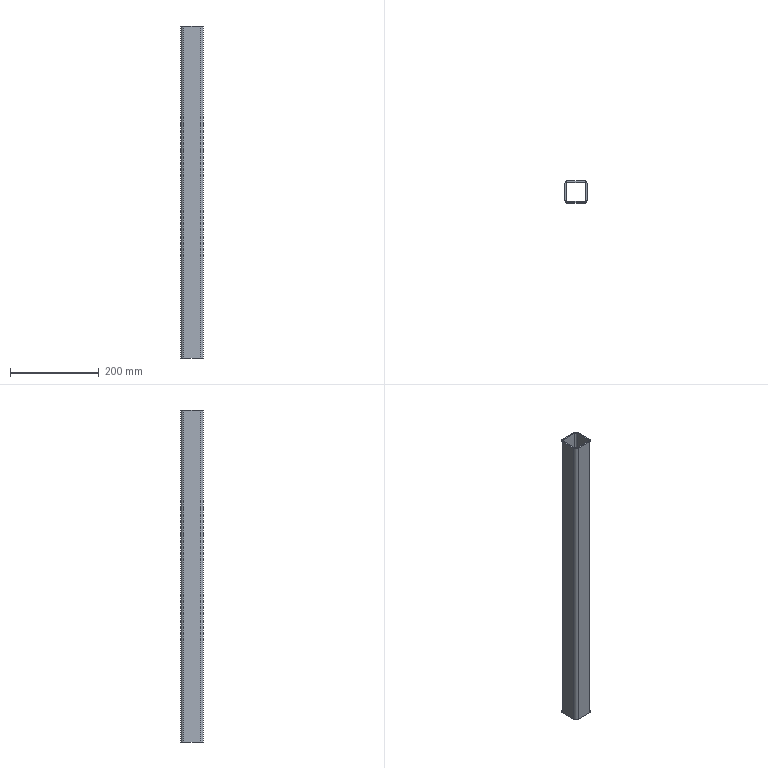Part | STEP file | JIS G 3466 50 x 50 x 3,2 1784903928658 | 1 solid | 18 faces | box 50 x 50 x 750 mm | volume 429502 mm3 | plane 10 | cylinder 8 | commonest cylinder face diameters 6.4 x4 12.8 x4
STEP:
#1=CARTESIAN_POINT('',(-18.6,-21.8,750.));
#2=VERTEX_POINT('',#1);
#3=CARTESIAN_POINT('',(18.6,-21.8,750.));
#4=VERTEX_POINT('',#3);
#5=CARTESIAN_POINT('',(9.3,-21.8,750.));
#6=DIRECTION('',(1.,0.,0.));
#7=VECTOR('',#6,10.);
#8=LINE('',#5,#7);
#9=EDGE_CURVE('',#2,#4,#8,.T.);
#10=ORIENTED_EDGE('',*,*,#9,.T.);
#11=CARTESIAN_POINT('',(18.6,-21.8,0.));
#12=VERTEX_POINT('',#11);
#13=CARTESIAN_POINT('',(18.6,-21.8,0.));
#14=DIRECTION('',(0.,0.,1.));
#15=VECTOR('',#14,10.);
#16=LINE('',#13,#15);
#17=EDGE_CURVE('',#12,#4,#16,.T.);
#18=ORIENTED_EDGE('',*,*,#17,.F.);
#19=CARTESIAN_POINT('',(-18.6,-21.8,0.));
#20=VERTEX_POINT('',#19);
#21=CARTESIAN_POINT('',(9.3,-21.8,0.));
#22=DIRECTION('',(1.,0.,0.));
#23=VECTOR('',#22,10.);
#24=LINE('',#21,#23);
#25=EDGE_CURVE('',#20,#12,#24,.T.);
#26=ORIENTED_EDGE('',*,*,#25,.F.);
#27=CARTESIAN_POINT('',(-18.6,-21.8,0.));
#28=DIRECTION('',(0.,0.,1.));
#29=VECTOR('',#28,10.);
#30=LINE('',#27,#29);
#31=EDGE_CURVE('',#20,#2,#30,.T.);
#32=ORIENTED_EDGE('',*,*,#31,.T.);
#33=EDGE_LOOP('',(#10,#18,#26,#32));
#34=FACE_OUTER_BOUND('',#33,.T.);
#35=CARTESIAN_POINT('',(18.6,-21.8,0.));
#36=DIRECTION('',(0.,-1.,0.));
#37=DIRECTION('',(0.,0.,-1.));
#38=AXIS2_PLACEMENT_3D('',#35,#36,#37);
#39=PLANE('',#38);
#40=ADVANCED_FACE('',(#34),#39,.F.);
#41=CARTESIAN_POINT('',(21.8,-18.6,750.));
#42=VERTEX_POINT('',#41);
#43=CARTESIAN_POINT('',(18.6,-18.6,750.));
#44=DIRECTION('',(0.,0.,1.));
#45=DIRECTION('',(0.,1.,0.));
#46=AXIS2_PLACEMENT_3D('',#43,#44,#45);
#47=CIRCLE('',#46,3.2);
#48=EDGE_CURVE('',#4,#42,#47,.T.);
#49=ORIENTED_EDGE('',*,*,#48,.T.);
#50=CARTESIAN_POINT('',(21.8,-18.6,0.));
#51=VERTEX_POINT('',#50);
#52=CARTESIAN_POINT('',(21.8,-18.6,0.));
#53=DIRECTION('',(0.,0.,1.));
#54=VECTOR('',#53,10.);
#55=LINE('',#52,#54);
#56=EDGE_CURVE('',#51,#42,#55,.T.);
#57=ORIENTED_EDGE('',*,*,#56,.F.);
#58=CARTESIAN_POINT('',(18.6,-18.6,0.));
#59=DIRECTION('',(0.,0.,1.));
#60=DIRECTION('',(0.,1.,0.));
#61=AXIS2_PLACEMENT_3D('',#58,#59,#60);
#62=CIRCLE('',#61,3.2);
#63=EDGE_CURVE('',#12,#51,#62,.T.);
#64=ORIENTED_EDGE('',*,*,#63,.F.);
#65=ORIENTED_EDGE('',*,*,#17,.T.);
#66=EDGE_LOOP('',(#49,#57,#64,#65));
#67=FACE_OUTER_BOUND('',#66,.T.);
#68=CARTESIAN_POINT('',(18.6,-18.6,0.));
#69=DIRECTION('',(0.,0.,1.));
#70=DIRECTION('',(0.,1.,0.));
#71=AXIS2_PLACEMENT_3D('',#68,#69,#70);
#72=CYLINDRICAL_SURFACE('',#71,3.2);
#73=ADVANCED_FACE('',(#67),#72,.F.);
#74=CARTESIAN_POINT('',(21.8,18.6,750.));
#75=VERTEX_POINT('',#74);
#76=CARTESIAN_POINT('',(21.8,9.3,750.));
#77=DIRECTION('',(0.,1.,0.));
#78=VECTOR('',#77,10.);
#79=LINE('',#76,#78);
#80=EDGE_CURVE('',#42,#75,#79,.T.);
#81=ORIENTED_EDGE('',*,*,#80,.T.);
#82=CARTESIAN_POINT('',(21.8,18.6,0.));
#83=VERTEX_POINT('',#82);
#84=CARTESIAN_POINT('',(21.8,18.6,0.));
#85=DIRECTION('',(0.,0.,1.));
#86=VECTOR('',#85,10.);
#87=LINE('',#84,#86);
#88=EDGE_CURVE('',#83,#75,#87,.T.);
#89=ORIENTED_EDGE('',*,*,#88,.F.);
#90=CARTESIAN_POINT('',(21.8,9.3,0.));
#91=DIRECTION('',(0.,1.,0.));
#92=VECTOR('',#91,10.);
#93=LINE('',#90,#92);
#94=EDGE_CURVE('',#51,#83,#93,.T.);
#95=ORIENTED_EDGE('',*,*,#94,.F.);
#96=ORIENTED_EDGE('',*,*,#56,.T.);
#97=EDGE_LOOP('',(#81,#89,#95,#96));
#98=FACE_OUTER_BOUND('',#97,.T.);
#99=CARTESIAN_POINT('',(21.8,18.6,0.));
#100=DIRECTION('',(1.,0.,0.));
#101=DIRECTION('',(0.,0.,-1.));
#102=AXIS2_PLACEMENT_3D('',#99,#100,#101);
#103=PLANE('',#102);
#104=ADVANCED_FACE('',(#98),#103,.F.);
#105=CARTESIAN_POINT('',(18.6,21.8,750.));
#106=VERTEX_POINT('',#105);
#107=CARTESIAN_POINT('',(18.6,18.6,750.));
#108=DIRECTION('',(0.,0.,1.));
#109=DIRECTION('',(-1.,0.,0.));
#110=AXIS2_PLACEMENT_3D('',#107,#108,#109);
#111=CIRCLE('',#110,3.2);
#112=EDGE_CURVE('',#75,#106,#111,.T.);
#113=ORIENTED_EDGE('',*,*,#112,.T.);
#114=CARTESIAN_POINT('',(18.6,21.8,0.));
#115=VERTEX_POINT('',#114);
#116=CARTESIAN_POINT('',(18.6,21.8,0.));
#117=DIRECTION('',(0.,0.,1.));
#118=VECTOR('',#117,10.);
#119=LINE('',#116,#118);
#120=EDGE_CURVE('',#115,#106,#119,.T.);
#121=ORIENTED_EDGE('',*,*,#120,.F.);
#122=CARTESIAN_POINT('',(18.6,18.6,0.));
#123=DIRECTION('',(0.,0.,1.));
#124=DIRECTION('',(-1.,0.,0.));
#125=AXIS2_PLACEMENT_3D('',#122,#123,#124);
#126=CIRCLE('',#125,3.2);
#127=EDGE_CURVE('',#83,#115,#126,.T.);
#128=ORIENTED_EDGE('',*,*,#127,.F.);
#129=ORIENTED_EDGE('',*,*,#88,.T.);
#130=EDGE_LOOP('',(#113,#121,#128,#129));
#131=FACE_OUTER_BOUND('',#130,.T.);
#132=CARTESIAN_POINT('',(18.6,18.6,0.));
#133=DIRECTION('',(0.,0.,1.));
#134=DIRECTION('',(-1.,0.,0.));
#135=AXIS2_PLACEMENT_3D('',#132,#133,#134);
#136=CYLINDRICAL_SURFACE('',#135,3.2);
#137=ADVANCED_FACE('',(#131),#136,.F.);
#138=CARTESIAN_POINT('',(25.,18.6,750.));
#139=VERTEX_POINT('',#138);
#140=CARTESIAN_POINT('',(25.,-18.6,750.));
#141=VERTEX_POINT('',#140);
#142=CARTESIAN_POINT('',(25.,9.3,750.));
#143=DIRECTION('',(0.,-1.,0.));
#144=VECTOR('',#143,10.);
#145=LINE('',#142,#144);
#146=EDGE_CURVE('',#139,#141,#145,.T.);
#147=ORIENTED_EDGE('',*,*,#146,.T.);
#148=CARTESIAN_POINT('',(25.,-18.6,0.));
#149=VERTEX_POINT('',#148);
#150=CARTESIAN_POINT('',(25.,-18.6,0.));
#151=DIRECTION('',(0.,0.,1.));
#152=VECTOR('',#151,10.);
#153=LINE('',#150,#152);
#154=EDGE_CURVE('',#149,#141,#153,.T.);
#155=ORIENTED_EDGE('',*,*,#154,.F.);
#156=CARTESIAN_POINT('',(25.,18.6,0.));
#157=VERTEX_POINT('',#156);
#158=CARTESIAN_POINT('',(25.,9.3,0.));
#159=DIRECTION('',(0.,-1.,0.));
#160=VECTOR('',#159,10.);
#161=LINE('',#158,#160);
#162=EDGE_CURVE('',#157,#149,#161,.T.);
#163=ORIENTED_EDGE('',*,*,#162,.F.);
#164=CARTESIAN_POINT('',(25.,18.6,0.));
#165=DIRECTION('',(0.,0.,1.));
#166=VECTOR('',#165,10.);
#167=LINE('',#164,#166);
#168=EDGE_CURVE('',#157,#139,#167,.T.);
#169=ORIENTED_EDGE('',*,*,#168,.T.);
#170=EDGE_LOOP('',(#147,#155,#163,#169));
#171=FACE_OUTER_BOUND('',#170,.T.);
#172=CARTESIAN_POINT('',(25.,18.6,0.));
#173=DIRECTION('',(1.,0.,0.));
#174=DIRECTION('',(0.,0.,-1.));
#175=AXIS2_PLACEMENT_3D('',#172,#173,#174);
#176=PLANE('',#175);
#177=ADVANCED_FACE('',(#171),#176,.T.);
#178=CARTESIAN_POINT('',(18.6,-25.,750.));
#179=VERTEX_POINT('',#178);
#180=CARTESIAN_POINT('',(18.6,-18.6,750.));
#181=DIRECTION('',(0.,0.,-1.));
#182=DIRECTION('',(0.,1.,0.));
#183=AXIS2_PLACEMENT_3D('',#180,#181,#182);
#184=CIRCLE('',#183,6.4);
#185=EDGE_CURVE('',#141,#179,#184,.T.);
#186=ORIENTED_EDGE('',*,*,#185,.T.);
#187=CARTESIAN_POINT('',(18.6,-25.,0.));
#188=VERTEX_POINT('',#187);
#189=CARTESIAN_POINT('',(18.6,-25.,0.));
#190=DIRECTION('',(0.,0.,1.));
#191=VECTOR('',#190,10.);
#192=LINE('',#189,#191);
#193=EDGE_CURVE('',#188,#179,#192,.T.);
#194=ORIENTED_EDGE('',*,*,#193,.F.);
#195=CARTESIAN_POINT('',(18.6,-18.6,0.));
#196=DIRECTION('',(0.,0.,-1.));
#197=DIRECTION('',(0.,1.,0.));
#198=AXIS2_PLACEMENT_3D('',#195,#196,#197);
#199=CIRCLE('',#198,6.4);
#200=EDGE_CURVE('',#149,#188,#199,.T.);
#201=ORIENTED_EDGE('',*,*,#200,.F.);
#202=ORIENTED_EDGE('',*,*,#154,.T.);
#203=EDGE_LOOP('',(#186,#194,#201,#202));
#204=FACE_OUTER_BOUND('',#203,.T.);
#205=CARTESIAN_POINT('',(18.6,-18.6,0.));
#206=DIRECTION('',(0.,0.,1.));
#207=DIRECTION('',(0.,1.,0.));
#208=AXIS2_PLACEMENT_3D('',#205,#206,#207);
#209=CYLINDRICAL_SURFACE('',#208,6.4);
#210=ADVANCED_FACE('',(#204),#209,.T.);
#211=CARTESIAN_POINT('',(-18.6,-25.,750.));
#212=VERTEX_POINT('',#211);
#213=CARTESIAN_POINT('',(9.3,-25.,750.));
#214=DIRECTION('',(-1.,0.,0.));
#215=VECTOR('',#214,10.);
#216=LINE('',#213,#215);
#217=EDGE_CURVE('',#179,#212,#216,.T.);
#218=ORIENTED_EDGE('',*,*,#217,.T.);
#219=CARTESIAN_POINT('',(-18.6,-25.,0.));
#220=VERTEX_POINT('',#219);
#221=CARTESIAN_POINT('',(-18.6,-25.,0.));
#222=DIRECTION('',(0.,0.,1.));
#223=VECTOR('',#222,10.);
#224=LINE('',#221,#223);
#225=EDGE_CURVE('',#220,#212,#224,.T.);
#226=ORIENTED_EDGE('',*,*,#225,.F.);
#227=CARTESIAN_POINT('',(9.3,-25.,0.));
#228=DIRECTION('',(-1.,0.,0.));
#229=VECTOR('',#228,10.);
#230=LINE('',#227,#229);
#231=EDGE_CURVE('',#188,#220,#230,.T.);
#232=ORIENTED_EDGE('',*,*,#231,.F.);
#233=ORIENTED_EDGE('',*,*,#193,.T.);
#234=EDGE_LOOP('',(#218,#226,#232,#233));
#235=FACE_OUTER_BOUND('',#234,.T.);
#236=CARTESIAN_POINT('',(18.6,-25.,0.));
#237=DIRECTION('',(0.,-1.,0.));
#238=DIRECTION('',(0.,0.,-1.));
#239=AXIS2_PLACEMENT_3D('',#236,#237,#238);
#240=PLANE('',#239);
#241=ADVANCED_FACE('',(#235),#240,.T.);
#242=CARTESIAN_POINT('',(-25.,-18.6,750.));
#243=VERTEX_POINT('',#242);
#244=CARTESIAN_POINT('',(-18.6,-18.6,750.));
#245=DIRECTION('',(0.,0.,-1.));
#246=DIRECTION('',(1.,0.,0.));
#247=AXIS2_PLACEMENT_3D('',#244,#245,#246);
#248=CIRCLE('',#247,6.4);
#249=EDGE_CURVE('',#212,#243,#248,.T.);
#250=ORIENTED_EDGE('',*,*,#249,.T.);
#251=CARTESIAN_POINT('',(-25.,-18.6,0.));
#252=VERTEX_POINT('',#251);
#253=CARTESIAN_POINT('',(-25.,-18.6,0.));
#254=DIRECTION('',(0.,0.,1.));
#255=VECTOR('',#254,10.);
#256=LINE('',#253,#255);
#257=EDGE_CURVE('',#252,#243,#256,.T.);
#258=ORIENTED_EDGE('',*,*,#257,.F.);
#259=CARTESIAN_POINT('',(-18.6,-18.6,0.));
#260=DIRECTION('',(0.,0.,-1.));
#261=DIRECTION('',(1.,0.,0.));
#262=AXIS2_PLACEMENT_3D('',#259,#260,#261);
#263=CIRCLE('',#262,6.4);
#264=EDGE_CURVE('',#220,#252,#263,.T.);
#265=ORIENTED_EDGE('',*,*,#264,.F.);
#266=ORIENTED_EDGE('',*,*,#225,.T.);
#267=EDGE_LOOP('',(#250,#258,#265,#266));
#268=FACE_OUTER_BOUND('',#267,.T.);
#269=CARTESIAN_POINT('',(-18.6,-18.6,0.));
#270=DIRECTION('',(0.,0.,1.));
#271=DIRECTION('',(1.,0.,0.));
#272=AXIS2_PLACEMENT_3D('',#269,#270,#271);
#273=CYLINDRICAL_SURFACE('',#272,6.4);
#274=ADVANCED_FACE('',(#268),#273,.T.);
#275=CARTESIAN_POINT('',(-18.6,21.8,750.));
#276=VERTEX_POINT('',#275);
#277=CARTESIAN_POINT('',(-9.3,21.8,750.));
#278=DIRECTION('',(-1.,0.,0.));
#279=VECTOR('',#278,10.);
#280=LINE('',#277,#279);
#281=EDGE_CURVE('',#106,#276,#280,.T.);
#282=ORIENTED_EDGE('',*,*,#281,.T.);
#283=CARTESIAN_POINT('',(-18.6,21.8,0.));
#284=VERTEX_POINT('',#283);
#285=CARTESIAN_POINT('',(-18.6,21.8,0.));
#286=DIRECTION('',(0.,0.,1.));
#287=VECTOR('',#286,10.);
#288=LINE('',#285,#287);
#289=EDGE_CURVE('',#284,#276,#288,.T.);
#290=ORIENTED_EDGE('',*,*,#289,.F.);
#291=CARTESIAN_POINT('',(-9.3,21.8,0.));
#292=DIRECTION('',(-1.,0.,0.));
#293=VECTOR('',#292,10.);
#294=LINE('',#291,#293);
#295=EDGE_CURVE('',#115,#284,#294,.T.);
#296=ORIENTED_EDGE('',*,*,#295,.F.);
#297=ORIENTED_EDGE('',*,*,#120,.T.);
#298=EDGE_LOOP('',(#282,#290,#296,#297));
#299=FACE_OUTER_BOUND('',#298,.T.);
#300=CARTESIAN_POINT('',(-18.6,21.8,0.));
#301=DIRECTION('',(0.,1.,0.));
#302=DIRECTION('',(0.,0.,1.));
#303=AXIS2_PLACEMENT_3D('',#300,#301,#302);
#304=PLANE('',#303);
#305=ADVANCED_FACE('',(#299),#304,.F.);
#306=CARTESIAN_POINT('',(-21.8,-18.6,750.));
#307=VERTEX_POINT('',#306);
#308=CARTESIAN_POINT('',(-18.6,-18.6,750.));
#309=DIRECTION('',(0.,0.,1.));
#310=DIRECTION('',(1.,0.,0.));
#311=AXIS2_PLACEMENT_3D('',#308,#309,#310);
#312=CIRCLE('',#311,3.2);
#313=EDGE_CURVE('',#307,#2,#312,.T.);
#314=ORIENTED_EDGE('',*,*,#313,.T.);
#315=ORIENTED_EDGE('',*,*,#31,.F.);
#316=CARTESIAN_POINT('',(-21.8,-18.6,0.));
#317=VERTEX_POINT('',#316);
#318=CARTESIAN_POINT('',(-18.6,-18.6,0.));
#319=DIRECTION('',(0.,0.,1.));
#320=DIRECTION('',(1.,0.,0.));
#321=AXIS2_PLACEMENT_3D('',#318,#319,#320);
#322=CIRCLE('',#321,3.2);
#323=EDGE_CURVE('',#317,#20,#322,.T.);
#324=ORIENTED_EDGE('',*,*,#323,.F.);
#325=CARTESIAN_POINT('',(-21.8,-18.6,0.));
#326=DIRECTION('',(0.,0.,1.));
#327=VECTOR('',#326,10.);
#328=LINE('',#325,#327);
#329=EDGE_CURVE('',#317,#307,#328,.T.);
#330=ORIENTED_EDGE('',*,*,#329,.T.);
#331=EDGE_LOOP('',(#314,#315,#324,#330));
#332=FACE_OUTER_BOUND('',#331,.T.);
#333=CARTESIAN_POINT('',(-18.6,-18.6,0.));
#334=DIRECTION('',(0.,0.,1.));
#335=DIRECTION('',(1.,0.,0.));
#336=AXIS2_PLACEMENT_3D('',#333,#334,#335);
#337=CYLINDRICAL_SURFACE('',#336,3.2);
#338=ADVANCED_FACE('',(#332),#337,.F.);
#339=CARTESIAN_POINT('',(-21.8,18.6,750.));
#340=VERTEX_POINT('',#339);
#341=CARTESIAN_POINT('',(-21.8,-9.3,750.));
#342=DIRECTION('',(0.,-1.,0.));
#343=VECTOR('',#342,10.);
#344=LINE('',#341,#343);
#345=EDGE_CURVE('',#340,#307,#344,.T.);
#346=ORIENTED_EDGE('',*,*,#345,.T.);
#347=ORIENTED_EDGE('',*,*,#329,.F.);
#348=CARTESIAN_POINT('',(-21.8,18.6,0.));
#349=VERTEX_POINT('',#348);
#350=CARTESIAN_POINT('',(-21.8,-9.3,0.));
#351=DIRECTION('',(0.,-1.,0.));
#352=VECTOR('',#351,10.);
#353=LINE('',#350,#352);
#354=EDGE_CURVE('',#349,#317,#353,.T.);
#355=ORIENTED_EDGE('',*,*,#354,.F.);
#356=CARTESIAN_POINT('',(-21.8,18.6,0.));
#357=DIRECTION('',(0.,0.,1.));
#358=VECTOR('',#357,10.);
#359=LINE('',#356,#358);
#360=EDGE_CURVE('',#349,#340,#359,.T.);
#361=ORIENTED_EDGE('',*,*,#360,.T.);
#362=EDGE_LOOP('',(#346,#347,#355,#361));
#363=FACE_OUTER_BOUND('',#362,.T.);
#364=CARTESIAN_POINT('',(-21.8,-18.6,0.));
#365=DIRECTION('',(-1.,0.,0.));
#366=DIRECTION('',(0.,0.,1.));
#367=AXIS2_PLACEMENT_3D('',#364,#365,#366);
#368=PLANE('',#367);
#369=ADVANCED_FACE('',(#363),#368,.F.);
#370=CARTESIAN_POINT('',(-18.6,18.6,750.));
#371=DIRECTION('',(0.,0.,1.));
#372=DIRECTION('',(0.,-1.,0.));
#373=AXIS2_PLACEMENT_3D('',#370,#371,#372);
#374=CIRCLE('',#373,3.2);
#375=EDGE_CURVE('',#276,#340,#374,.T.);
#376=ORIENTED_EDGE('',*,*,#375,.T.);
#377=ORIENTED_EDGE('',*,*,#360,.F.);
#378=CARTESIAN_POINT('',(-18.6,18.6,0.));
#379=DIRECTION('',(0.,0.,1.));
#380=DIRECTION('',(0.,-1.,0.));
#381=AXIS2_PLACEMENT_3D('',#378,#379,#380);
#382=CIRCLE('',#381,3.2);
#383=EDGE_CURVE('',#284,#349,#382,.T.);
#384=ORIENTED_EDGE('',*,*,#383,.F.);
#385=ORIENTED_EDGE('',*,*,#289,.T.);
#386=EDGE_LOOP('',(#376,#377,#384,#385));
#387=FACE_OUTER_BOUND('',#386,.T.);
#388=CARTESIAN_POINT('',(-18.6,18.6,0.));
#389=DIRECTION('',(0.,0.,1.));
#390=DIRECTION('',(0.,-1.,0.));
#391=AXIS2_PLACEMENT_3D('',#388,#389,#390);
#392=CYLINDRICAL_SURFACE('',#391,3.2);
#393=ADVANCED_FACE('',(#387),#392,.F.);
#394=CARTESIAN_POINT('',(-25.,18.6,750.));
#395=VERTEX_POINT('',#394);
#396=CARTESIAN_POINT('',(-25.,-9.3,750.));
#397=DIRECTION('',(0.,1.,0.));
#398=VECTOR('',#397,10.);
#399=LINE('',#396,#398);
#400=EDGE_CURVE('',#243,#395,#399,.T.);
#401=ORIENTED_EDGE('',*,*,#400,.T.);
#402=CARTESIAN_POINT('',(-25.,18.6,0.));
#403=VERTEX_POINT('',#402);
#404=CARTESIAN_POINT('',(-25.,18.6,0.));
#405=DIRECTION('',(0.,0.,1.));
#406=VECTOR('',#405,10.);
#407=LINE('',#404,#406);
#408=EDGE_CURVE('',#403,#395,#407,.T.);
#409=ORIENTED_EDGE('',*,*,#408,.F.);
#410=CARTESIAN_POINT('',(-25.,-9.3,0.));
#411=DIRECTION('',(0.,1.,0.));
#412=VECTOR('',#411,10.);
#413=LINE('',#410,#412);
#414=EDGE_CURVE('',#252,#403,#413,.T.);
#415=ORIENTED_EDGE('',*,*,#414,.F.);
#416=ORIENTED_EDGE('',*,*,#257,.T.);
#417=EDGE_LOOP('',(#401,#409,#415,#416));
#418=FACE_OUTER_BOUND('',#417,.T.);
#419=CARTESIAN_POINT('',(-25.,-18.6,0.));
#420=DIRECTION('',(-1.,0.,0.));
#421=DIRECTION('',(0.,0.,1.));
#422=AXIS2_PLACEMENT_3D('',#419,#420,#421);
#423=PLANE('',#422);
#424=ADVANCED_FACE('',(#418),#423,.T.);
#425=CARTESIAN_POINT('',(-18.6,25.,750.));
#426=VERTEX_POINT('',#425);
#427=CARTESIAN_POINT('',(-18.6,18.6,750.));
#428=DIRECTION('',(0.,0.,-1.));
#429=DIRECTION('',(0.,-1.,0.));
#430=AXIS2_PLACEMENT_3D('',#427,#428,#429);
#431=CIRCLE('',#430,6.4);
#432=EDGE_CURVE('',#395,#426,#431,.T.);
#433=ORIENTED_EDGE('',*,*,#432,.T.);
#434=CARTESIAN_POINT('',(-18.6,25.,0.));
#435=VERTEX_POINT('',#434);
#436=CARTESIAN_POINT('',(-18.6,25.,0.));
#437=DIRECTION('',(0.,0.,1.));
#438=VECTOR('',#437,10.);
#439=LINE('',#436,#438);
#440=EDGE_CURVE('',#435,#426,#439,.T.);
#441=ORIENTED_EDGE('',*,*,#440,.F.);
#442=CARTESIAN_POINT('',(-18.6,18.6,0.));
#443=DIRECTION('',(0.,0.,-1.));
#444=DIRECTION('',(0.,-1.,0.));
#445=AXIS2_PLACEMENT_3D('',#442,#443,#444);
#446=CIRCLE('',#445,6.4);
#447=EDGE_CURVE('',#403,#435,#446,.T.);
#448=ORIENTED_EDGE('',*,*,#447,.F.);
#449=ORIENTED_EDGE('',*,*,#408,.T.);
#450=EDGE_LOOP('',(#433,#441,#448,#449));
#451=FACE_OUTER_BOUND('',#450,.T.);
#452=CARTESIAN_POINT('',(-18.6,18.6,0.));
#453=DIRECTION('',(0.,0.,1.));
#454=DIRECTION('',(0.,-1.,0.));
#455=AXIS2_PLACEMENT_3D('',#452,#453,#454);
#456=CYLINDRICAL_SURFACE('',#455,6.4);
#457=ADVANCED_FACE('',(#451),#456,.T.);
#458=CARTESIAN_POINT('',(18.6,25.,750.));
#459=VERTEX_POINT('',#458);
#460=CARTESIAN_POINT('',(-9.3,25.,750.));
#461=DIRECTION('',(1.,0.,0.));
#462=VECTOR('',#461,10.);
#463=LINE('',#460,#462);
#464=EDGE_CURVE('',#426,#459,#463,.T.);
#465=ORIENTED_EDGE('',*,*,#464,.T.);
#466=CARTESIAN_POINT('',(18.6,25.,0.));
#467=VERTEX_POINT('',#466);
#468=CARTESIAN_POINT('',(18.6,25.,0.));
#469=DIRECTION('',(0.,0.,1.));
#470=VECTOR('',#469,10.);
#471=LINE('',#468,#470);
#472=EDGE_CURVE('',#467,#459,#471,.T.);
#473=ORIENTED_EDGE('',*,*,#472,.F.);
#474=CARTESIAN_POINT('',(-9.3,25.,0.));
#475=DIRECTION('',(1.,0.,0.));
#476=VECTOR('',#475,10.);
#477=LINE('',#474,#476);
#478=EDGE_CURVE('',#435,#467,#477,.T.);
#479=ORIENTED_EDGE('',*,*,#478,.F.);
#480=ORIENTED_EDGE('',*,*,#440,.T.);
#481=EDGE_LOOP('',(#465,#473,#479,#480));
#482=FACE_OUTER_BOUND('',#481,.T.);
#483=CARTESIAN_POINT('',(-18.6,25.,0.));
#484=DIRECTION('',(0.,1.,0.));
#485=DIRECTION('',(0.,0.,1.));
#486=AXIS2_PLACEMENT_3D('',#483,#484,#485);
#487=PLANE('',#486);
#488=ADVANCED_FACE('',(#482),#487,.T.);
#489=CARTESIAN_POINT('',(18.6,18.6,750.));
#490=DIRECTION('',(0.,0.,-1.));
#491=DIRECTION('',(-1.,0.,0.));
#492=AXIS2_PLACEMENT_3D('',#489,#490,#491);
#493=CIRCLE('',#492,6.4);
#494=EDGE_CURVE('',#459,#139,#493,.T.);
#495=ORIENTED_EDGE('',*,*,#494,.T.);
#496=ORIENTED_EDGE('',*,*,#168,.F.);
#497=CARTESIAN_POINT('',(18.6,18.6,0.));
#498=DIRECTION('',(0.,0.,-1.));
#499=DIRECTION('',(-1.,0.,0.));
#500=AXIS2_PLACEMENT_3D('',#497,#498,#499);
#501=CIRCLE('',#500,6.4);
#502=EDGE_CURVE('',#467,#157,#501,.T.);
#503=ORIENTED_EDGE('',*,*,#502,.F.);
#504=ORIENTED_EDGE('',*,*,#472,.T.);
#505=EDGE_LOOP('',(#495,#496,#503,#504));
#506=FACE_OUTER_BOUND('',#505,.T.);
#507=CARTESIAN_POINT('',(18.6,18.6,0.));
#508=DIRECTION('',(0.,0.,1.));
#509=DIRECTION('',(-1.,0.,0.));
#510=AXIS2_PLACEMENT_3D('',#507,#508,#509);
#511=CYLINDRICAL_SURFACE('',#510,6.4);
#512=ADVANCED_FACE('',(#506),#511,.T.);
#513=ORIENTED_EDGE('',*,*,#414,.T.);
#514=ORIENTED_EDGE('',*,*,#447,.T.);
#515=ORIENTED_EDGE('',*,*,#478,.T.);
#516=ORIENTED_EDGE('',*,*,#502,.T.);
#517=ORIENTED_EDGE('',*,*,#162,.T.);
#518=ORIENTED_EDGE('',*,*,#200,.T.);
#519=ORIENTED_EDGE('',*,*,#231,.T.);
#520=ORIENTED_EDGE('',*,*,#264,.T.);
#521=EDGE_LOOP('',(#513,#514,#515,#516,#517,#518,#519,#520));
#522=FACE_OUTER_BOUND('',#521,.T.);
#523=ORIENTED_EDGE('',*,*,#295,.T.);
#524=ORIENTED_EDGE('',*,*,#383,.T.);
#525=ORIENTED_EDGE('',*,*,#354,.T.);
#526=ORIENTED_EDGE('',*,*,#323,.T.);
#527=ORIENTED_EDGE('',*,*,#25,.T.);
#528=ORIENTED_EDGE('',*,*,#63,.T.);
#529=ORIENTED_EDGE('',*,*,#94,.T.);
#530=ORIENTED_EDGE('',*,*,#127,.T.);
#531=EDGE_LOOP('',(#523,#524,#525,#526,#527,#528,#529,#530));
#532=FACE_BOUND('',#531,.T.);
#533=CARTESIAN_POINT('',(0.,0.,0.));
#534=DIRECTION('',(0.,0.,1.));
#535=DIRECTION('',(1.,0.,0.));
#536=AXIS2_PLACEMENT_3D('',#533,#534,#535);
#537=PLANE('',#536);
#538=ADVANCED_FACE('',(#522,#532),#537,.F.);
#539=ORIENTED_EDGE('',*,*,#400,.F.);
#540=ORIENTED_EDGE('',*,*,#249,.F.);
#541=ORIENTED_EDGE('',*,*,#217,.F.);
#542=ORIENTED_EDGE('',*,*,#185,.F.);
#543=ORIENTED_EDGE('',*,*,#146,.F.);
#544=ORIENTED_EDGE('',*,*,#494,.F.);
#545=ORIENTED_EDGE('',*,*,#464,.F.);
#546=ORIENTED_EDGE('',*,*,#432,.F.);
#547=EDGE_LOOP('',(#539,#540,#541,#542,#543,#544,#545,#546));
#548=FACE_OUTER_BOUND('',#547,.T.);
#549=ORIENTED_EDGE('',*,*,#281,.F.);
#550=ORIENTED_EDGE('',*,*,#112,.F.);
#551=ORIENTED_EDGE('',*,*,#80,.F.);
#552=ORIENTED_EDGE('',*,*,#48,.F.);
#553=ORIENTED_EDGE('',*,*,#9,.F.);
#554=ORIENTED_EDGE('',*,*,#313,.F.);
#555=ORIENTED_EDGE('',*,*,#345,.F.);
#556=ORIENTED_EDGE('',*,*,#375,.F.);
#557=EDGE_LOOP('',(#549,#550,#551,#552,#553,#554,#555,#556));
#558=FACE_BOUND('',#557,.T.);
#559=CARTESIAN_POINT('',(0.,0.,750.));
#560=DIRECTION('',(0.,0.,1.));
#561=DIRECTION('',(1.,0.,0.));
#562=AXIS2_PLACEMENT_3D('',#559,#560,#561);
#563=PLANE('',#562);
#564=ADVANCED_FACE('',(#548,#558),#563,.T.);
#565=CLOSED_SHELL('',(#40,#73,#104,#137,#177,#210,#241,#274,#305,#338,#369,#393,#424,#457,#488,#512,#538,#564));
#566=MANIFOLD_SOLID_BREP('',#565);
#567=(LENGTH_UNIT()NAMED_UNIT(*)SI_UNIT(.MILLI.,.METRE.));
#568=UNCERTAINTY_MEASURE_WITH_UNIT(LENGTH_MEASURE(0.01),#567,'','');
#569=(NAMED_UNIT(*)PLANE_ANGLE_UNIT()SI_UNIT($,.RADIAN.));
#570=(NAMED_UNIT(*)SI_UNIT($,.STERADIAN.)SOLID_ANGLE_UNIT());
#571=(GEOMETRIC_REPRESENTATION_CONTEXT(3)GLOBAL_UNCERTAINTY_ASSIGNED_CONTEXT((#568))GLOBAL_UNIT_ASSIGNED_CONTEXT((#567,#569,#570))REPRESENTATION_CONTEXT('',''));
#572=ADVANCED_BREP_SHAPE_REPRESENTATION('',(#566),#571);